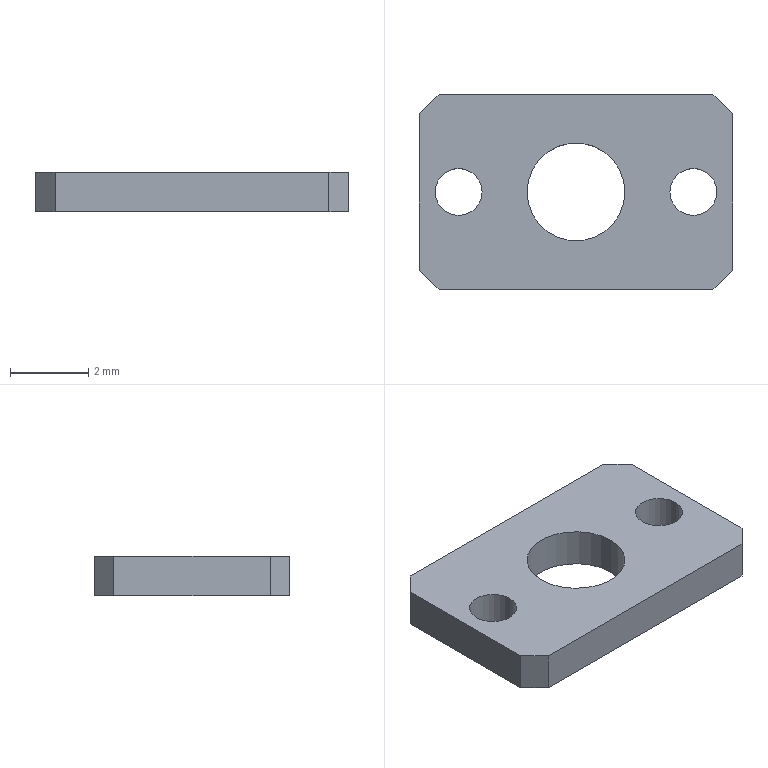Part | SolidWorks | features Chamfer 1, Extrusion 1, ICE 1 | 1 solid | 16 faces | box 8 x 5 x 1 mm | volume 32.329 mm3 | plane 10 | cylinder 6 | commonest cylinder face diameters 1.2 x4 2.5 x2
STEP:
#1=CARTESIAN_POINT('',(2.4,0.,-0.5));
#2=VERTEX_POINT('',#1);
#3=CARTESIAN_POINT('',(3.6,0.,-0.5));
#4=VERTEX_POINT('',#3);
#5=CARTESIAN_POINT('',(3.,0.,-0.5));
#6=DIRECTION('',(0.,0.,1.));
#7=DIRECTION('',(1.,0.,0.));
#8=AXIS2_PLACEMENT_3D('',#5,#6,#7);
#9=CIRCLE('',#8,0.6);
#10=EDGE_CURVE('',#2,#4,#9,.T.);
#11=ORIENTED_EDGE('',*,*,#10,.F.);
#12=CARTESIAN_POINT('',(2.4,0.,0.5));
#13=VERTEX_POINT('',#12);
#14=CARTESIAN_POINT('',(2.4,0.,-0.5));
#15=DIRECTION('',(0.,0.,1.));
#16=VECTOR('',#15,1000.);
#17=LINE('',#14,#16);
#18=EDGE_CURVE('',#2,#13,#17,.T.);
#19=ORIENTED_EDGE('',*,*,#18,.T.);
#20=CARTESIAN_POINT('',(3.6,0.,0.5));
#21=VERTEX_POINT('',#20);
#22=CARTESIAN_POINT('',(3.,0.,0.5));
#23=DIRECTION('',(0.,0.,1.));
#24=DIRECTION('',(1.,0.,0.));
#25=AXIS2_PLACEMENT_3D('',#22,#23,#24);
#26=CIRCLE('',#25,0.6);
#27=EDGE_CURVE('',#13,#21,#26,.T.);
#28=ORIENTED_EDGE('',*,*,#27,.T.);
#29=CARTESIAN_POINT('',(3.6,0.,-0.5));
#30=DIRECTION('',(0.,0.,1.));
#31=VECTOR('',#30,1000.);
#32=LINE('',#29,#31);
#33=EDGE_CURVE('',#4,#21,#32,.T.);
#34=ORIENTED_EDGE('',*,*,#33,.F.);
#35=EDGE_LOOP('',(#11,#19,#28,#34));
#36=FACE_OUTER_BOUND('',#35,.T.);
#37=CARTESIAN_POINT('',(3.,0.,-0.5));
#38=DIRECTION('',(0.,0.,1.));
#39=DIRECTION('',(1.,0.,0.));
#40=AXIS2_PLACEMENT_3D('',#37,#38,#39);
#41=CYLINDRICAL_SURFACE('',#40,0.6);
#42=ADVANCED_FACE('',(#36),#41,.F.);
#43=CARTESIAN_POINT('',(-3.6,0.,-0.5));
#44=VERTEX_POINT('',#43);
#45=CARTESIAN_POINT('',(-2.4,0.,-0.5));
#46=VERTEX_POINT('',#45);
#47=CARTESIAN_POINT('',(-3.,0.,-0.5));
#48=DIRECTION('',(0.,0.,1.));
#49=DIRECTION('',(1.,0.,0.));
#50=AXIS2_PLACEMENT_3D('',#47,#48,#49);
#51=CIRCLE('',#50,0.6);
#52=EDGE_CURVE('',#44,#46,#51,.T.);
#53=ORIENTED_EDGE('',*,*,#52,.F.);
#54=CARTESIAN_POINT('',(-3.6,0.,0.5));
#55=VERTEX_POINT('',#54);
#56=CARTESIAN_POINT('',(-3.6,0.,-0.5));
#57=DIRECTION('',(0.,0.,1.));
#58=VECTOR('',#57,1000.);
#59=LINE('',#56,#58);
#60=EDGE_CURVE('',#44,#55,#59,.T.);
#61=ORIENTED_EDGE('',*,*,#60,.T.);
#62=CARTESIAN_POINT('',(-2.4,0.,0.5));
#63=VERTEX_POINT('',#62);
#64=CARTESIAN_POINT('',(-3.,0.,0.5));
#65=DIRECTION('',(0.,0.,1.));
#66=DIRECTION('',(1.,0.,0.));
#67=AXIS2_PLACEMENT_3D('',#64,#65,#66);
#68=CIRCLE('',#67,0.6);
#69=EDGE_CURVE('',#55,#63,#68,.T.);
#70=ORIENTED_EDGE('',*,*,#69,.T.);
#71=CARTESIAN_POINT('',(-2.4,0.,-0.5));
#72=DIRECTION('',(0.,0.,1.));
#73=VECTOR('',#72,1000.);
#74=LINE('',#71,#73);
#75=EDGE_CURVE('',#46,#63,#74,.T.);
#76=ORIENTED_EDGE('',*,*,#75,.F.);
#77=EDGE_LOOP('',(#53,#61,#70,#76));
#78=FACE_OUTER_BOUND('',#77,.T.);
#79=CARTESIAN_POINT('',(-3.,0.,-0.5));
#80=DIRECTION('',(0.,0.,1.));
#81=DIRECTION('',(1.,0.,0.));
#82=AXIS2_PLACEMENT_3D('',#79,#80,#81);
#83=CYLINDRICAL_SURFACE('',#82,0.6);
#84=ADVANCED_FACE('',(#78),#83,.F.);
#85=CARTESIAN_POINT('',(-1.25,0.,-0.5));
#86=VERTEX_POINT('',#85);
#87=CARTESIAN_POINT('',(1.25,0.,-0.5));
#88=VERTEX_POINT('',#87);
#89=CARTESIAN_POINT('',(0.,0.,-0.5));
#90=DIRECTION('',(0.,0.,1.));
#91=DIRECTION('',(1.,0.,0.));
#92=AXIS2_PLACEMENT_3D('',#89,#90,#91);
#93=CIRCLE('',#92,1.25);
#94=EDGE_CURVE('',#86,#88,#93,.T.);
#95=ORIENTED_EDGE('',*,*,#94,.F.);
#96=CARTESIAN_POINT('',(-1.25,0.,0.5));
#97=VERTEX_POINT('',#96);
#98=CARTESIAN_POINT('',(-1.25,0.,-0.5));
#99=DIRECTION('',(0.,0.,1.));
#100=VECTOR('',#99,1000.);
#101=LINE('',#98,#100);
#102=EDGE_CURVE('',#86,#97,#101,.T.);
#103=ORIENTED_EDGE('',*,*,#102,.T.);
#104=CARTESIAN_POINT('',(1.25,0.,0.5));
#105=VERTEX_POINT('',#104);
#106=CARTESIAN_POINT('',(0.,0.,0.5));
#107=DIRECTION('',(0.,0.,1.));
#108=DIRECTION('',(1.,0.,0.));
#109=AXIS2_PLACEMENT_3D('',#106,#107,#108);
#110=CIRCLE('',#109,1.25);
#111=EDGE_CURVE('',#97,#105,#110,.T.);
#112=ORIENTED_EDGE('',*,*,#111,.T.);
#113=CARTESIAN_POINT('',(1.25,0.,-0.5));
#114=DIRECTION('',(0.,0.,1.));
#115=VECTOR('',#114,1000.);
#116=LINE('',#113,#115);
#117=EDGE_CURVE('',#88,#105,#116,.T.);
#118=ORIENTED_EDGE('',*,*,#117,.F.);
#119=EDGE_LOOP('',(#95,#103,#112,#118));
#120=FACE_OUTER_BOUND('',#119,.T.);
#121=CARTESIAN_POINT('',(0.,0.,-0.5));
#122=DIRECTION('',(0.,0.,1.));
#123=DIRECTION('',(1.,0.,0.));
#124=AXIS2_PLACEMENT_3D('',#121,#122,#123);
#125=CYLINDRICAL_SURFACE('',#124,1.25);
#126=ADVANCED_FACE('',(#120),#125,.F.);
#127=CARTESIAN_POINT('',(4.,-2.,0.5));
#128=VERTEX_POINT('',#127);
#129=CARTESIAN_POINT('',(4.,2.,0.5));
#130=VERTEX_POINT('',#129);
#131=CARTESIAN_POINT('',(4.,2.5,0.5));
#132=DIRECTION('',(0.,1.,0.));
#133=VECTOR('',#132,1000.);
#134=LINE('',#131,#133);
#135=EDGE_CURVE('',#128,#130,#134,.T.);
#136=ORIENTED_EDGE('',*,*,#135,.F.);
#137=CARTESIAN_POINT('',(4.,-2.,-0.5));
#138=VERTEX_POINT('',#137);
#139=CARTESIAN_POINT('',(4.,-2.,0.5));
#140=DIRECTION('',(0.,0.,-1.));
#141=VECTOR('',#140,1000.);
#142=LINE('',#139,#141);
#143=EDGE_CURVE('',#128,#138,#142,.T.);
#144=ORIENTED_EDGE('',*,*,#143,.T.);
#145=CARTESIAN_POINT('',(4.,2.,-0.5));
#146=VERTEX_POINT('',#145);
#147=CARTESIAN_POINT('',(4.,2.5,-0.5));
#148=DIRECTION('',(0.,1.,0.));
#149=VECTOR('',#148,1000.);
#150=LINE('',#147,#149);
#151=EDGE_CURVE('',#138,#146,#150,.T.);
#152=ORIENTED_EDGE('',*,*,#151,.T.);
#153=CARTESIAN_POINT('',(4.,2.,0.5));
#154=DIRECTION('',(0.,0.,1.));
#155=VECTOR('',#154,1000.);
#156=LINE('',#153,#155);
#157=EDGE_CURVE('',#146,#130,#156,.T.);
#158=ORIENTED_EDGE('',*,*,#157,.T.);
#159=EDGE_LOOP('',(#136,#144,#152,#158));
#160=FACE_OUTER_BOUND('',#159,.T.);
#161=CARTESIAN_POINT('',(4.,2.5,0.5));
#162=DIRECTION('',(-1.,0.,0.));
#163=DIRECTION('',(0.,-1.,0.));
#164=AXIS2_PLACEMENT_3D('',#161,#162,#163);
#165=PLANE('',#164);
#166=ADVANCED_FACE('',(#160),#165,.F.);
#167=CARTESIAN_POINT('',(3.5,2.5,-0.5));
#168=VERTEX_POINT('',#167);
#169=CARTESIAN_POINT('',(-3.5,2.5,-0.5));
#170=VERTEX_POINT('',#169);
#171=CARTESIAN_POINT('',(-4.,2.5,-0.5));
#172=DIRECTION('',(-1.,0.,0.));
#173=VECTOR('',#172,1000.);
#174=LINE('',#171,#173);
#175=EDGE_CURVE('',#168,#170,#174,.T.);
#176=ORIENTED_EDGE('',*,*,#175,.T.);
#177=CARTESIAN_POINT('',(-3.5,2.5,0.5));
#178=VERTEX_POINT('',#177);
#179=CARTESIAN_POINT('',(-3.5,2.5,0.5));
#180=DIRECTION('',(0.,0.,1.));
#181=VECTOR('',#180,1000.);
#182=LINE('',#179,#181);
#183=EDGE_CURVE('',#170,#178,#182,.T.);
#184=ORIENTED_EDGE('',*,*,#183,.T.);
#185=CARTESIAN_POINT('',(3.5,2.5,0.5));
#186=VERTEX_POINT('',#185);
#187=CARTESIAN_POINT('',(-4.,2.5,0.5));
#188=DIRECTION('',(-1.,0.,0.));
#189=VECTOR('',#188,1000.);
#190=LINE('',#187,#189);
#191=EDGE_CURVE('',#186,#178,#190,.T.);
#192=ORIENTED_EDGE('',*,*,#191,.F.);
#193=CARTESIAN_POINT('',(3.5,2.5,0.5));
#194=DIRECTION('',(0.,0.,-1.));
#195=VECTOR('',#194,1000.);
#196=LINE('',#193,#195);
#197=EDGE_CURVE('',#186,#168,#196,.T.);
#198=ORIENTED_EDGE('',*,*,#197,.T.);
#199=EDGE_LOOP('',(#176,#184,#192,#198));
#200=FACE_OUTER_BOUND('',#199,.T.);
#201=CARTESIAN_POINT('',(-4.,2.5,0.5));
#202=DIRECTION('',(0.,-1.,0.));
#203=DIRECTION('',(0.,0.,-1.));
#204=AXIS2_PLACEMENT_3D('',#201,#202,#203);
#205=PLANE('',#204);
#206=ADVANCED_FACE('',(#200),#205,.F.);
#207=CARTESIAN_POINT('',(-4.,2.,-0.5));
#208=VERTEX_POINT('',#207);
#209=CARTESIAN_POINT('',(-4.,-2.,-0.5));
#210=VERTEX_POINT('',#209);
#211=CARTESIAN_POINT('',(-4.,2.5,-0.5));
#212=DIRECTION('',(0.,-1.,0.));
#213=VECTOR('',#212,1000.);
#214=LINE('',#211,#213);
#215=EDGE_CURVE('',#208,#210,#214,.T.);
#216=ORIENTED_EDGE('',*,*,#215,.T.);
#217=CARTESIAN_POINT('',(-4.,-2.,0.5));
#218=VERTEX_POINT('',#217);
#219=CARTESIAN_POINT('',(-4.,-2.,0.5));
#220=DIRECTION('',(0.,0.,1.));
#221=VECTOR('',#220,1000.);
#222=LINE('',#219,#221);
#223=EDGE_CURVE('',#210,#218,#222,.T.);
#224=ORIENTED_EDGE('',*,*,#223,.T.);
#225=CARTESIAN_POINT('',(-4.,2.,0.5));
#226=VERTEX_POINT('',#225);
#227=CARTESIAN_POINT('',(-4.,2.5,0.5));
#228=DIRECTION('',(0.,-1.,0.));
#229=VECTOR('',#228,1000.);
#230=LINE('',#227,#229);
#231=EDGE_CURVE('',#226,#218,#230,.T.);
#232=ORIENTED_EDGE('',*,*,#231,.F.);
#233=CARTESIAN_POINT('',(-4.,2.,0.5));
#234=DIRECTION('',(0.,0.,-1.));
#235=VECTOR('',#234,1000.);
#236=LINE('',#233,#235);
#237=EDGE_CURVE('',#226,#208,#236,.T.);
#238=ORIENTED_EDGE('',*,*,#237,.T.);
#239=EDGE_LOOP('',(#216,#224,#232,#238));
#240=FACE_OUTER_BOUND('',#239,.T.);
#241=CARTESIAN_POINT('',(-4.,2.5,0.5));
#242=DIRECTION('',(1.,0.,0.));
#243=DIRECTION('',(0.,1.,0.));
#244=AXIS2_PLACEMENT_3D('',#241,#242,#243);
#245=PLANE('',#244);
#246=ADVANCED_FACE('',(#240),#245,.F.);
#247=CARTESIAN_POINT('',(-3.5,-2.5,0.5));
#248=VERTEX_POINT('',#247);
#249=CARTESIAN_POINT('',(3.5,-2.5,0.5));
#250=VERTEX_POINT('',#249);
#251=CARTESIAN_POINT('',(-4.,-2.5,0.5));
#252=DIRECTION('',(1.,0.,0.));
#253=VECTOR('',#252,1000.);
#254=LINE('',#251,#253);
#255=EDGE_CURVE('',#248,#250,#254,.T.);
#256=ORIENTED_EDGE('',*,*,#255,.F.);
#257=CARTESIAN_POINT('',(-3.5,-2.5,-0.5));
#258=VERTEX_POINT('',#257);
#259=CARTESIAN_POINT('',(-3.5,-2.5,0.5));
#260=DIRECTION('',(0.,0.,-1.));
#261=VECTOR('',#260,1000.);
#262=LINE('',#259,#261);
#263=EDGE_CURVE('',#248,#258,#262,.T.);
#264=ORIENTED_EDGE('',*,*,#263,.T.);
#265=CARTESIAN_POINT('',(3.5,-2.5,-0.5));
#266=VERTEX_POINT('',#265);
#267=CARTESIAN_POINT('',(-4.,-2.5,-0.5));
#268=DIRECTION('',(1.,0.,0.));
#269=VECTOR('',#268,1000.);
#270=LINE('',#267,#269);
#271=EDGE_CURVE('',#258,#266,#270,.T.);
#272=ORIENTED_EDGE('',*,*,#271,.T.);
#273=CARTESIAN_POINT('',(3.5,-2.5,0.5));
#274=DIRECTION('',(0.,0.,1.));
#275=VECTOR('',#274,1000.);
#276=LINE('',#273,#275);
#277=EDGE_CURVE('',#266,#250,#276,.T.);
#278=ORIENTED_EDGE('',*,*,#277,.T.);
#279=EDGE_LOOP('',(#256,#264,#272,#278));
#280=FACE_OUTER_BOUND('',#279,.T.);
#281=CARTESIAN_POINT('',(-4.,-2.5,0.5));
#282=DIRECTION('',(0.,1.,0.));
#283=DIRECTION('',(0.,0.,1.));
#284=AXIS2_PLACEMENT_3D('',#281,#282,#283);
#285=PLANE('',#284);
#286=ADVANCED_FACE('',(#280),#285,.F.);
#287=CARTESIAN_POINT('',(3.,0.,0.5));
#288=DIRECTION('',(0.,0.,1.));
#289=DIRECTION('',(1.,0.,0.));
#290=AXIS2_PLACEMENT_3D('',#287,#288,#289);
#291=CIRCLE('',#290,0.6);
#292=EDGE_CURVE('',#21,#13,#291,.T.);
#293=ORIENTED_EDGE('',*,*,#292,.F.);
#294=ORIENTED_EDGE('',*,*,#27,.F.);
#295=EDGE_LOOP('',(#293,#294));
#296=FACE_BOUND('',#295,.T.);
#297=CARTESIAN_POINT('',(-3.,0.,0.5));
#298=DIRECTION('',(0.,0.,1.));
#299=DIRECTION('',(1.,0.,0.));
#300=AXIS2_PLACEMENT_3D('',#297,#298,#299);
#301=CIRCLE('',#300,0.6);
#302=EDGE_CURVE('',#63,#55,#301,.T.);
#303=ORIENTED_EDGE('',*,*,#302,.F.);
#304=ORIENTED_EDGE('',*,*,#69,.F.);
#305=EDGE_LOOP('',(#303,#304));
#306=FACE_BOUND('',#305,.T.);
#307=CARTESIAN_POINT('',(0.,0.,0.5));
#308=DIRECTION('',(0.,0.,1.));
#309=DIRECTION('',(1.,0.,0.));
#310=AXIS2_PLACEMENT_3D('',#307,#308,#309);
#311=CIRCLE('',#310,1.25);
#312=EDGE_CURVE('',#105,#97,#311,.T.);
#313=ORIENTED_EDGE('',*,*,#312,.F.);
#314=ORIENTED_EDGE('',*,*,#111,.F.);
#315=EDGE_LOOP('',(#313,#314));
#316=FACE_BOUND('',#315,.T.);
#317=ORIENTED_EDGE('',*,*,#231,.T.);
#318=CARTESIAN_POINT('',(-3.,-3.,0.5));
#319=DIRECTION('',(0.7071,-0.7071,0.));
#320=VECTOR('',#319,1000.);
#321=LINE('',#318,#320);
#322=EDGE_CURVE('',#218,#248,#321,.T.);
#323=ORIENTED_EDGE('',*,*,#322,.T.);
#324=ORIENTED_EDGE('',*,*,#255,.T.);
#325=CARTESIAN_POINT('',(3.,-3.,0.5));
#326=DIRECTION('',(0.7071,0.7071,0.));
#327=VECTOR('',#326,1000.);
#328=LINE('',#325,#327);
#329=EDGE_CURVE('',#250,#128,#328,.T.);
#330=ORIENTED_EDGE('',*,*,#329,.T.);
#331=ORIENTED_EDGE('',*,*,#135,.T.);
#332=CARTESIAN_POINT('',(3.,3.,0.5));
#333=DIRECTION('',(-0.7071,0.7071,0.));
#334=VECTOR('',#333,1000.);
#335=LINE('',#332,#334);
#336=EDGE_CURVE('',#130,#186,#335,.T.);
#337=ORIENTED_EDGE('',*,*,#336,.T.);
#338=ORIENTED_EDGE('',*,*,#191,.T.);
#339=CARTESIAN_POINT('',(-3.,3.,0.5));
#340=DIRECTION('',(-0.7071,-0.7071,0.));
#341=VECTOR('',#340,1000.);
#342=LINE('',#339,#341);
#343=EDGE_CURVE('',#178,#226,#342,.T.);
#344=ORIENTED_EDGE('',*,*,#343,.T.);
#345=EDGE_LOOP('',(#317,#323,#324,#330,#331,#337,#338,#344));
#346=FACE_OUTER_BOUND('',#345,.T.);
#347=CARTESIAN_POINT('',(0.,0.,0.5));
#348=DIRECTION('',(0.,0.,1.));
#349=DIRECTION('',(1.,0.,0.));
#350=AXIS2_PLACEMENT_3D('',#347,#348,#349);
#351=PLANE('',#350);
#352=ADVANCED_FACE('',(#296,#306,#316,#346),#351,.T.);
#353=CARTESIAN_POINT('',(3.,0.,-0.5));
#354=DIRECTION('',(0.,0.,1.));
#355=DIRECTION('',(1.,0.,0.));
#356=AXIS2_PLACEMENT_3D('',#353,#354,#355);
#357=CIRCLE('',#356,0.6);
#358=EDGE_CURVE('',#4,#2,#357,.T.);
#359=ORIENTED_EDGE('',*,*,#358,.T.);
#360=ORIENTED_EDGE('',*,*,#10,.T.);
#361=EDGE_LOOP('',(#359,#360));
#362=FACE_BOUND('',#361,.T.);
#363=CARTESIAN_POINT('',(-3.,0.,-0.5));
#364=DIRECTION('',(0.,0.,1.));
#365=DIRECTION('',(1.,0.,0.));
#366=AXIS2_PLACEMENT_3D('',#363,#364,#365);
#367=CIRCLE('',#366,0.6);
#368=EDGE_CURVE('',#46,#44,#367,.T.);
#369=ORIENTED_EDGE('',*,*,#368,.T.);
#370=ORIENTED_EDGE('',*,*,#52,.T.);
#371=EDGE_LOOP('',(#369,#370));
#372=FACE_BOUND('',#371,.T.);
#373=CARTESIAN_POINT('',(0.,0.,-0.5));
#374=DIRECTION('',(0.,0.,1.));
#375=DIRECTION('',(1.,0.,0.));
#376=AXIS2_PLACEMENT_3D('',#373,#374,#375);
#377=CIRCLE('',#376,1.25);
#378=EDGE_CURVE('',#88,#86,#377,.T.);
#379=ORIENTED_EDGE('',*,*,#378,.T.);
#380=ORIENTED_EDGE('',*,*,#94,.T.);
#381=EDGE_LOOP('',(#379,#380));
#382=FACE_BOUND('',#381,.T.);
#383=ORIENTED_EDGE('',*,*,#271,.F.);
#384=CARTESIAN_POINT('',(-3.5,-2.5,-0.5));
#385=DIRECTION('',(-0.7071,0.7071,0.));
#386=VECTOR('',#385,1000.);
#387=LINE('',#384,#386);
#388=EDGE_CURVE('',#258,#210,#387,.T.);
#389=ORIENTED_EDGE('',*,*,#388,.T.);
#390=ORIENTED_EDGE('',*,*,#215,.F.);
#391=CARTESIAN_POINT('',(-4.,2.,-0.5));
#392=DIRECTION('',(0.7071,0.7071,0.));
#393=VECTOR('',#392,1000.);
#394=LINE('',#391,#393);
#395=EDGE_CURVE('',#208,#170,#394,.T.);
#396=ORIENTED_EDGE('',*,*,#395,.T.);
#397=ORIENTED_EDGE('',*,*,#175,.F.);
#398=CARTESIAN_POINT('',(3.5,2.5,-0.5));
#399=DIRECTION('',(0.7071,-0.7071,0.));
#400=VECTOR('',#399,1000.);
#401=LINE('',#398,#400);
#402=EDGE_CURVE('',#168,#146,#401,.T.);
#403=ORIENTED_EDGE('',*,*,#402,.T.);
#404=ORIENTED_EDGE('',*,*,#151,.F.);
#405=CARTESIAN_POINT('',(4.,-2.,-0.5));
#406=DIRECTION('',(-0.7071,-0.7071,0.));
#407=VECTOR('',#406,1000.);
#408=LINE('',#405,#407);
#409=EDGE_CURVE('',#138,#266,#408,.T.);
#410=ORIENTED_EDGE('',*,*,#409,.T.);
#411=EDGE_LOOP('',(#383,#389,#390,#396,#397,#403,#404,#410));
#412=FACE_OUTER_BOUND('',#411,.T.);
#413=CARTESIAN_POINT('',(0.,0.,-0.5));
#414=DIRECTION('',(0.,0.,1.));
#415=DIRECTION('',(1.,0.,0.));
#416=AXIS2_PLACEMENT_3D('',#413,#414,#415);
#417=PLANE('',#416);
#418=ADVANCED_FACE('',(#362,#372,#382,#412),#417,.F.);
#419=ORIENTED_EDGE('',*,*,#102,.F.);
#420=ORIENTED_EDGE('',*,*,#378,.F.);
#421=ORIENTED_EDGE('',*,*,#117,.T.);
#422=ORIENTED_EDGE('',*,*,#312,.T.);
#423=EDGE_LOOP('',(#419,#420,#421,#422));
#424=FACE_OUTER_BOUND('',#423,.T.);
#425=CARTESIAN_POINT('',(0.,0.,-0.5));
#426=DIRECTION('',(0.,0.,1.));
#427=DIRECTION('',(1.,0.,0.));
#428=AXIS2_PLACEMENT_3D('',#425,#426,#427);
#429=CYLINDRICAL_SURFACE('',#428,1.25);
#430=ADVANCED_FACE('',(#424),#429,.F.);
#431=ORIENTED_EDGE('',*,*,#60,.F.);
#432=ORIENTED_EDGE('',*,*,#368,.F.);
#433=ORIENTED_EDGE('',*,*,#75,.T.);
#434=ORIENTED_EDGE('',*,*,#302,.T.);
#435=EDGE_LOOP('',(#431,#432,#433,#434));
#436=FACE_OUTER_BOUND('',#435,.T.);
#437=CARTESIAN_POINT('',(-3.,0.,-0.5));
#438=DIRECTION('',(0.,0.,1.));
#439=DIRECTION('',(1.,0.,0.));
#440=AXIS2_PLACEMENT_3D('',#437,#438,#439);
#441=CYLINDRICAL_SURFACE('',#440,0.6);
#442=ADVANCED_FACE('',(#436),#441,.F.);
#443=ORIENTED_EDGE('',*,*,#18,.F.);
#444=ORIENTED_EDGE('',*,*,#358,.F.);
#445=ORIENTED_EDGE('',*,*,#33,.T.);
#446=ORIENTED_EDGE('',*,*,#292,.T.);
#447=EDGE_LOOP('',(#443,#444,#445,#446));
#448=FACE_OUTER_BOUND('',#447,.T.);
#449=CARTESIAN_POINT('',(3.,0.,-0.5));
#450=DIRECTION('',(0.,0.,1.));
#451=DIRECTION('',(1.,0.,0.));
#452=AXIS2_PLACEMENT_3D('',#449,#450,#451);
#453=CYLINDRICAL_SURFACE('',#452,0.6);
#454=ADVANCED_FACE('',(#448),#453,.F.);
#455=ORIENTED_EDGE('',*,*,#322,.F.);
#456=ORIENTED_EDGE('',*,*,#223,.F.);
#457=ORIENTED_EDGE('',*,*,#388,.F.);
#458=ORIENTED_EDGE('',*,*,#263,.F.);
#459=EDGE_LOOP('',(#455,#456,#457,#458));
#460=FACE_OUTER_BOUND('',#459,.T.);
#461=CARTESIAN_POINT('',(-3.5,-2.5,0.5));
#462=DIRECTION('',(0.7071,0.7071,0.));
#463=DIRECTION('',(0.,0.,-1.));
#464=AXIS2_PLACEMENT_3D('',#461,#462,#463);
#465=PLANE('',#464);
#466=ADVANCED_FACE('',(#460),#465,.F.);
#467=ORIENTED_EDGE('',*,*,#343,.F.);
#468=ORIENTED_EDGE('',*,*,#183,.F.);
#469=ORIENTED_EDGE('',*,*,#395,.F.);
#470=ORIENTED_EDGE('',*,*,#237,.F.);
#471=EDGE_LOOP('',(#467,#468,#469,#470));
#472=FACE_OUTER_BOUND('',#471,.T.);
#473=CARTESIAN_POINT('',(-4.,2.,0.5));
#474=DIRECTION('',(0.7071,-0.7071,0.));
#475=DIRECTION('',(0.,0.,-1.));
#476=AXIS2_PLACEMENT_3D('',#473,#474,#475);
#477=PLANE('',#476);
#478=ADVANCED_FACE('',(#472),#477,.F.);
#479=ORIENTED_EDGE('',*,*,#329,.F.);
#480=ORIENTED_EDGE('',*,*,#277,.F.);
#481=ORIENTED_EDGE('',*,*,#409,.F.);
#482=ORIENTED_EDGE('',*,*,#143,.F.);
#483=EDGE_LOOP('',(#479,#480,#481,#482));
#484=FACE_OUTER_BOUND('',#483,.T.);
#485=CARTESIAN_POINT('',(4.,-2.,0.5));
#486=DIRECTION('',(-0.7071,0.7071,0.));
#487=DIRECTION('',(0.,0.,-1.));
#488=AXIS2_PLACEMENT_3D('',#485,#486,#487);
#489=PLANE('',#488);
#490=ADVANCED_FACE('',(#484),#489,.F.);
#491=ORIENTED_EDGE('',*,*,#336,.F.);
#492=ORIENTED_EDGE('',*,*,#157,.F.);
#493=ORIENTED_EDGE('',*,*,#402,.F.);
#494=ORIENTED_EDGE('',*,*,#197,.F.);
#495=EDGE_LOOP('',(#491,#492,#493,#494));
#496=FACE_OUTER_BOUND('',#495,.T.);
#497=CARTESIAN_POINT('',(3.5,2.5,0.5));
#498=DIRECTION('',(-0.7071,-0.7071,0.));
#499=DIRECTION('',(0.,0.,-1.));
#500=AXIS2_PLACEMENT_3D('',#497,#498,#499);
#501=PLANE('',#500);
#502=ADVANCED_FACE('',(#496),#501,.F.);
#503=CLOSED_SHELL('',(#42,#84,#126,#166,#206,#246,#286,#352,#418,#430,#442,#454,#466,#478,#490,#502));
#504=MANIFOLD_SOLID_BREP('',#503);
#505=CARTESIAN_POINT('',(0.,0.,0.));
#506=DIRECTION('',(0.,0.,1.));
#507=DIRECTION('',(1.,0.,0.));
#508=AXIS2_PLACEMENT_3D('',#505,#506,#507);
#509=(LENGTH_UNIT()NAMED_UNIT(*)SI_UNIT(.MILLI.,.METRE.));
#510=UNCERTAINTY_MEASURE_WITH_UNIT(LENGTH_MEASURE(0.00001),#509,'','');
#511=(NAMED_UNIT(*)PLANE_ANGLE_UNIT()SI_UNIT($,.RADIAN.));
#512=(NAMED_UNIT(*)SI_UNIT($,.STERADIAN.)SOLID_ANGLE_UNIT());
#513=(GEOMETRIC_REPRESENTATION_CONTEXT(3)GLOBAL_UNCERTAINTY_ASSIGNED_CONTEXT((#510))GLOBAL_UNIT_ASSIGNED_CONTEXT((#509,#511,#512))REPRESENTATION_CONTEXT('',''));
#514=ADVANCED_BREP_SHAPE_REPRESENTATION('',(#504,#508),#513);